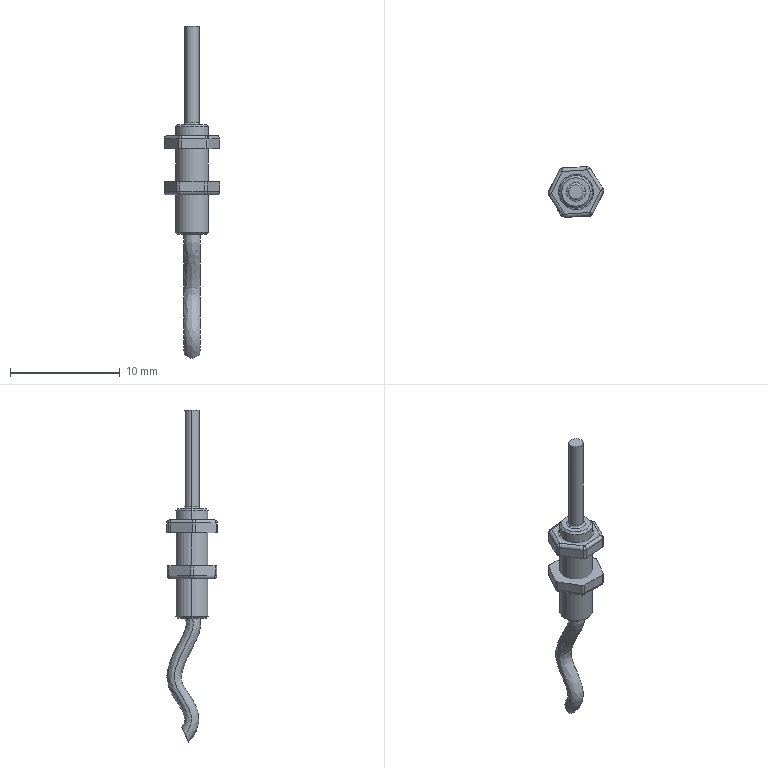Part | NX | features BREP 3 | 3 solids | 78 faces | box 5.103 x 4.647 x 30.276 mm | volume 128.594 mm3 | cylinder 32 | plane 20 | sphere 14 | torus 6 | cone 4 | spline 2 | commonest cylinder face diameters 0.6 x24 2.6 x4 1.3 x2 3 x2